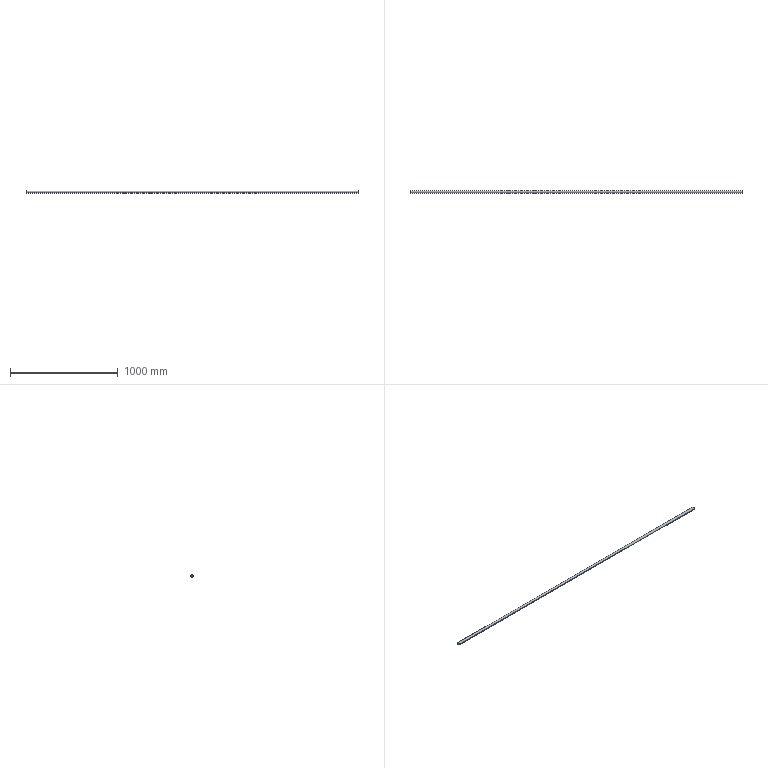Part | STEP file | 电柜护栏2栏杆_Default<As Machined> | 1 solid | 6 faces | box 3080 x 25 x 25 mm | volume 341083 mm3 | cylinder 4 | plane 2 | commonest cylinder face diameters 22 x2 25 x2
STEP:
#1=CARTESIAN_POINT('',(0.,0.,0.));
#2=DIRECTION('',(0.,0.,1.));
#3=DIRECTION('',(1.,0.,0.));
#4=AXIS2_PLACEMENT_3D('',#1,#2,#3);
#5=CARTESIAN_POINT('',(1540.,12.5,0.));
#6=VERTEX_POINT('',#5);
#7=CARTESIAN_POINT('',(1540.,-12.5,0.));
#8=VERTEX_POINT('',#7);
#9=CARTESIAN_POINT('',(1540.,0.,0.));
#10=DIRECTION('',(1.,0.,0.));
#11=DIRECTION('',(0.,1.,0.));
#12=AXIS2_PLACEMENT_3D('',#9,#10,#11);
#13=CIRCLE('',#12,12.5);
#14=CARTESIAN_POINT('',(1540.,0.,0.));
#15=DIRECTION('',(-1.,0.,0.));
#16=DIRECTION('',(0.,-1.,0.));
#17=AXIS2_PLACEMENT_3D('',#14,#15,#16);
#18=CYLINDRICAL_SURFACE('',#17,12.5);
#19=CARTESIAN_POINT('',(3.142,0.));
#20=DIRECTION('',(-1.,0.));
#21=VECTOR('',#20,1.);
#22=LINE('',#19,#21);
#23=(GEOMETRIC_REPRESENTATION_CONTEXT(2)PARAMETRIC_REPRESENTATION_CONTEXT()REPRESENTATION_CONTEXT('',''));
#24=DEFINITIONAL_REPRESENTATION('',(#22),#23);
#25=PCURVE('',#18,#24);
#26=CARTESIAN_POINT('',(1540.,0.,0.));
#27=DIRECTION('',(1.,0.,0.));
#28=DIRECTION('',(0.,1.,0.));
#29=AXIS2_PLACEMENT_3D('',#26,#27,#28);
#30=PLANE('',#29);
#31=CARTESIAN_POINT('',(0.,0.));
#32=DIRECTION('',(1.,0.));
#33=AXIS2_PLACEMENT_2D('',#31,#32);
#34=CIRCLE('',#33,12.5);
#35=(GEOMETRIC_REPRESENTATION_CONTEXT(2)PARAMETRIC_REPRESENTATION_CONTEXT()REPRESENTATION_CONTEXT('',''));
#36=DEFINITIONAL_REPRESENTATION('',(#34),#35);
#37=PCURVE('',#30,#36);
#38=SURFACE_CURVE('',#13,(#25,#37),.PCURVE_S1.);
#39=EDGE_CURVE('',#6,#8,#38,.T.);
#40=ORIENTED_EDGE('',*,*,#39,.F.);
#41=CARTESIAN_POINT('',(-1540.,12.5,0.));
#42=VERTEX_POINT('',#41);
#43=CARTESIAN_POINT('',(1540.,12.5,0.));
#44=DIRECTION('',(-1.,0.,0.));
#45=VECTOR('',#44,1.);
#46=LINE('',#43,#45);
#47=CARTESIAN_POINT('',(3.142,0.));
#48=DIRECTION('',(0.,1.));
#49=VECTOR('',#48,1.);
#50=LINE('',#47,#49);
#51=(GEOMETRIC_REPRESENTATION_CONTEXT(2)PARAMETRIC_REPRESENTATION_CONTEXT()REPRESENTATION_CONTEXT('',''));
#52=DEFINITIONAL_REPRESENTATION('',(#50),#51);
#53=PCURVE('',#18,#52);
#54=CARTESIAN_POINT('',(1540.,0.,0.));
#55=DIRECTION('',(-1.,0.,0.));
#56=DIRECTION('',(0.,-1.,0.));
#57=AXIS2_PLACEMENT_3D('',#54,#55,#56);
#58=CYLINDRICAL_SURFACE('',#57,12.5);
#59=CARTESIAN_POINT('',(3.142,0.));
#60=DIRECTION('',(0.,1.));
#61=VECTOR('',#60,1.);
#62=LINE('',#59,#61);
#63=(GEOMETRIC_REPRESENTATION_CONTEXT(2)PARAMETRIC_REPRESENTATION_CONTEXT()REPRESENTATION_CONTEXT('',''));
#64=DEFINITIONAL_REPRESENTATION('',(#62),#63);
#65=PCURVE('',#58,#64);
#66=SURFACE_CURVE('',#46,(#53,#65),.PCURVE_S1.);
#67=EDGE_CURVE('',#6,#42,#66,.T.);
#68=ORIENTED_EDGE('',*,*,#67,.T.);
#69=CARTESIAN_POINT('',(-1540.,-12.5,0.));
#70=VERTEX_POINT('',#69);
#71=CARTESIAN_POINT('',(-1540.,0.,0.));
#72=DIRECTION('',(1.,0.,0.));
#73=DIRECTION('',(0.,1.,0.));
#74=AXIS2_PLACEMENT_3D('',#71,#72,#73);
#75=CIRCLE('',#74,12.5);
#76=CARTESIAN_POINT('',(3.142,3080.));
#77=DIRECTION('',(-1.,0.));
#78=VECTOR('',#77,1.);
#79=LINE('',#76,#78);
#80=(GEOMETRIC_REPRESENTATION_CONTEXT(2)PARAMETRIC_REPRESENTATION_CONTEXT()REPRESENTATION_CONTEXT('',''));
#81=DEFINITIONAL_REPRESENTATION('',(#79),#80);
#82=PCURVE('',#18,#81);
#83=CARTESIAN_POINT('',(-1540.,0.,0.));
#84=DIRECTION('',(1.,0.,0.));
#85=DIRECTION('',(0.,1.,0.));
#86=AXIS2_PLACEMENT_3D('',#83,#84,#85);
#87=PLANE('',#86);
#88=CARTESIAN_POINT('',(0.,0.));
#89=DIRECTION('',(1.,0.));
#90=AXIS2_PLACEMENT_2D('',#88,#89);
#91=CIRCLE('',#90,12.5);
#92=(GEOMETRIC_REPRESENTATION_CONTEXT(2)PARAMETRIC_REPRESENTATION_CONTEXT()REPRESENTATION_CONTEXT('',''));
#93=DEFINITIONAL_REPRESENTATION('',(#91),#92);
#94=PCURVE('',#87,#93);
#95=SURFACE_CURVE('',#75,(#82,#94),.PCURVE_S1.);
#96=EDGE_CURVE('',#42,#70,#95,.T.);
#97=ORIENTED_EDGE('',*,*,#96,.T.);
#98=CARTESIAN_POINT('',(1540.,-12.5,0.));
#99=DIRECTION('',(-1.,0.,0.));
#100=VECTOR('',#99,1.);
#101=LINE('',#98,#100);
#102=CARTESIAN_POINT('',(0.,0.));
#103=DIRECTION('',(0.,1.));
#104=VECTOR('',#103,1.);
#105=LINE('',#102,#104);
#106=(GEOMETRIC_REPRESENTATION_CONTEXT(2)PARAMETRIC_REPRESENTATION_CONTEXT()REPRESENTATION_CONTEXT('',''));
#107=DEFINITIONAL_REPRESENTATION('',(#105),#106);
#108=PCURVE('',#18,#107);
#109=CARTESIAN_POINT('',(6.283,0.));
#110=DIRECTION('',(0.,1.));
#111=VECTOR('',#110,1.);
#112=LINE('',#109,#111);
#113=(GEOMETRIC_REPRESENTATION_CONTEXT(2)PARAMETRIC_REPRESENTATION_CONTEXT()REPRESENTATION_CONTEXT('',''));
#114=DEFINITIONAL_REPRESENTATION('',(#112),#113);
#115=PCURVE('',#58,#114);
#116=SURFACE_CURVE('',#101,(#108,#115),.PCURVE_S1.);
#117=EDGE_CURVE('',#8,#70,#116,.T.);
#118=ORIENTED_EDGE('',*,*,#117,.F.);
#119=EDGE_LOOP('',(#40,#68,#97,#118));
#120=FACE_BOUND('',#119,.T.);
#121=ADVANCED_FACE('',(#120),#18,.T.);
#122=CARTESIAN_POINT('',(1540.,-11.,0.));
#123=VERTEX_POINT('',#122);
#124=CARTESIAN_POINT('',(-1540.,-11.,0.));
#125=VERTEX_POINT('',#124);
#126=CARTESIAN_POINT('',(1540.,-11.,0.));
#127=DIRECTION('',(-1.,0.,0.));
#128=VECTOR('',#127,1.);
#129=LINE('',#126,#128);
#130=CARTESIAN_POINT('',(1540.,0.,0.));
#131=DIRECTION('',(-1.,0.,0.));
#132=DIRECTION('',(0.,-1.,0.));
#133=AXIS2_PLACEMENT_3D('',#130,#131,#132);
#134=CYLINDRICAL_SURFACE('',#133,11.);
#135=CARTESIAN_POINT('',(6.283,0.));
#136=DIRECTION('',(0.,1.));
#137=VECTOR('',#136,1.);
#138=LINE('',#135,#137);
#139=(GEOMETRIC_REPRESENTATION_CONTEXT(2)PARAMETRIC_REPRESENTATION_CONTEXT()REPRESENTATION_CONTEXT('',''));
#140=DEFINITIONAL_REPRESENTATION('',(#138),#139);
#141=PCURVE('',#134,#140);
#142=CARTESIAN_POINT('',(1540.,0.,0.));
#143=DIRECTION('',(-1.,0.,0.));
#144=DIRECTION('',(0.,-1.,0.));
#145=AXIS2_PLACEMENT_3D('',#142,#143,#144);
#146=CYLINDRICAL_SURFACE('',#145,11.);
#147=CARTESIAN_POINT('',(0.,0.));
#148=DIRECTION('',(0.,1.));
#149=VECTOR('',#148,1.);
#150=LINE('',#147,#149);
#151=(GEOMETRIC_REPRESENTATION_CONTEXT(2)PARAMETRIC_REPRESENTATION_CONTEXT()REPRESENTATION_CONTEXT('',''));
#152=DEFINITIONAL_REPRESENTATION('',(#150),#151);
#153=PCURVE('',#146,#152);
#154=SURFACE_CURVE('',#129,(#141,#153),.PCURVE_S1.);
#155=EDGE_CURVE('',#123,#125,#154,.T.);
#156=ORIENTED_EDGE('',*,*,#155,.T.);
#157=CARTESIAN_POINT('',(-1540.,11.,0.));
#158=VERTEX_POINT('',#157);
#159=CARTESIAN_POINT('',(-1540.,0.,0.));
#160=DIRECTION('',(1.,0.,0.));
#161=DIRECTION('',(0.,1.,0.));
#162=AXIS2_PLACEMENT_3D('',#159,#160,#161);
#163=CIRCLE('',#162,11.);
#164=CARTESIAN_POINT('',(9.425,3080.));
#165=DIRECTION('',(-1.,0.));
#166=VECTOR('',#165,1.);
#167=LINE('',#164,#166);
#168=(GEOMETRIC_REPRESENTATION_CONTEXT(2)PARAMETRIC_REPRESENTATION_CONTEXT()REPRESENTATION_CONTEXT('',''));
#169=DEFINITIONAL_REPRESENTATION('',(#167),#168);
#170=PCURVE('',#134,#169);
#171=CARTESIAN_POINT('',(0.,0.));
#172=DIRECTION('',(1.,0.));
#173=AXIS2_PLACEMENT_2D('',#171,#172);
#174=CIRCLE('',#173,11.);
#175=(GEOMETRIC_REPRESENTATION_CONTEXT(2)PARAMETRIC_REPRESENTATION_CONTEXT()REPRESENTATION_CONTEXT('',''));
#176=DEFINITIONAL_REPRESENTATION('',(#174),#175);
#177=PCURVE('',#87,#176);
#178=SURFACE_CURVE('',#163,(#170,#177),.PCURVE_S1.);
#179=EDGE_CURVE('',#125,#158,#178,.T.);
#180=ORIENTED_EDGE('',*,*,#179,.T.);
#181=CARTESIAN_POINT('',(1540.,11.,0.));
#182=VERTEX_POINT('',#181);
#183=CARTESIAN_POINT('',(1540.,11.,0.));
#184=DIRECTION('',(-1.,0.,0.));
#185=VECTOR('',#184,1.);
#186=LINE('',#183,#185);
#187=CARTESIAN_POINT('',(3.142,0.));
#188=DIRECTION('',(0.,1.));
#189=VECTOR('',#188,1.);
#190=LINE('',#187,#189);
#191=(GEOMETRIC_REPRESENTATION_CONTEXT(2)PARAMETRIC_REPRESENTATION_CONTEXT()REPRESENTATION_CONTEXT('',''));
#192=DEFINITIONAL_REPRESENTATION('',(#190),#191);
#193=PCURVE('',#134,#192);
#194=CARTESIAN_POINT('',(3.142,0.));
#195=DIRECTION('',(0.,1.));
#196=VECTOR('',#195,1.);
#197=LINE('',#194,#196);
#198=(GEOMETRIC_REPRESENTATION_CONTEXT(2)PARAMETRIC_REPRESENTATION_CONTEXT()REPRESENTATION_CONTEXT('',''));
#199=DEFINITIONAL_REPRESENTATION('',(#197),#198);
#200=PCURVE('',#146,#199);
#201=SURFACE_CURVE('',#186,(#193,#200),.PCURVE_S1.);
#202=EDGE_CURVE('',#182,#158,#201,.T.);
#203=ORIENTED_EDGE('',*,*,#202,.F.);
#204=CARTESIAN_POINT('',(1540.,0.,0.));
#205=DIRECTION('',(1.,0.,0.));
#206=DIRECTION('',(0.,1.,0.));
#207=AXIS2_PLACEMENT_3D('',#204,#205,#206);
#208=CIRCLE('',#207,11.);
#209=CARTESIAN_POINT('',(9.425,0.));
#210=DIRECTION('',(-1.,0.));
#211=VECTOR('',#210,1.);
#212=LINE('',#209,#211);
#213=(GEOMETRIC_REPRESENTATION_CONTEXT(2)PARAMETRIC_REPRESENTATION_CONTEXT()REPRESENTATION_CONTEXT('',''));
#214=DEFINITIONAL_REPRESENTATION('',(#212),#213);
#215=PCURVE('',#134,#214);
#216=CARTESIAN_POINT('',(0.,0.));
#217=DIRECTION('',(1.,0.));
#218=AXIS2_PLACEMENT_2D('',#216,#217);
#219=CIRCLE('',#218,11.);
#220=(GEOMETRIC_REPRESENTATION_CONTEXT(2)PARAMETRIC_REPRESENTATION_CONTEXT()REPRESENTATION_CONTEXT('',''));
#221=DEFINITIONAL_REPRESENTATION('',(#219),#220);
#222=PCURVE('',#30,#221);
#223=SURFACE_CURVE('',#208,(#215,#222),.PCURVE_S1.);
#224=EDGE_CURVE('',#123,#182,#223,.T.);
#225=ORIENTED_EDGE('',*,*,#224,.F.);
#226=EDGE_LOOP('',(#156,#180,#203,#225));
#227=FACE_BOUND('',#226,.F.);
#228=ADVANCED_FACE('',(#227),#134,.F.);
#229=CARTESIAN_POINT('',(-1540.,0.,0.));
#230=DIRECTION('',(1.,0.,0.));
#231=DIRECTION('',(0.,1.,0.));
#232=AXIS2_PLACEMENT_3D('',#229,#230,#231);
#233=CIRCLE('',#232,11.);
#234=CARTESIAN_POINT('',(3.142,3080.));
#235=DIRECTION('',(-1.,0.));
#236=VECTOR('',#235,1.);
#237=LINE('',#234,#236);
#238=(GEOMETRIC_REPRESENTATION_CONTEXT(2)PARAMETRIC_REPRESENTATION_CONTEXT()REPRESENTATION_CONTEXT('',''));
#239=DEFINITIONAL_REPRESENTATION('',(#237),#238);
#240=PCURVE('',#146,#239);
#241=CARTESIAN_POINT('',(0.,0.));
#242=DIRECTION('',(1.,0.));
#243=AXIS2_PLACEMENT_2D('',#241,#242);
#244=CIRCLE('',#243,11.);
#245=(GEOMETRIC_REPRESENTATION_CONTEXT(2)PARAMETRIC_REPRESENTATION_CONTEXT()REPRESENTATION_CONTEXT('',''));
#246=DEFINITIONAL_REPRESENTATION('',(#244),#245);
#247=PCURVE('',#87,#246);
#248=SURFACE_CURVE('',#233,(#240,#247),.PCURVE_S1.);
#249=EDGE_CURVE('',#158,#125,#248,.T.);
#250=ORIENTED_EDGE('',*,*,#249,.T.);
#251=ORIENTED_EDGE('',*,*,#155,.F.);
#252=CARTESIAN_POINT('',(1540.,0.,0.));
#253=DIRECTION('',(1.,0.,0.));
#254=DIRECTION('',(0.,1.,0.));
#255=AXIS2_PLACEMENT_3D('',#252,#253,#254);
#256=CIRCLE('',#255,11.);
#257=CARTESIAN_POINT('',(3.142,0.));
#258=DIRECTION('',(-1.,0.));
#259=VECTOR('',#258,1.);
#260=LINE('',#257,#259);
#261=(GEOMETRIC_REPRESENTATION_CONTEXT(2)PARAMETRIC_REPRESENTATION_CONTEXT()REPRESENTATION_CONTEXT('',''));
#262=DEFINITIONAL_REPRESENTATION('',(#260),#261);
#263=PCURVE('',#146,#262);
#264=CARTESIAN_POINT('',(0.,0.));
#265=DIRECTION('',(1.,0.));
#266=AXIS2_PLACEMENT_2D('',#264,#265);
#267=CIRCLE('',#266,11.);
#268=(GEOMETRIC_REPRESENTATION_CONTEXT(2)PARAMETRIC_REPRESENTATION_CONTEXT()REPRESENTATION_CONTEXT('',''));
#269=DEFINITIONAL_REPRESENTATION('',(#267),#268);
#270=PCURVE('',#30,#269);
#271=SURFACE_CURVE('',#256,(#263,#270),.PCURVE_S1.);
#272=EDGE_CURVE('',#182,#123,#271,.T.);
#273=ORIENTED_EDGE('',*,*,#272,.F.);
#274=ORIENTED_EDGE('',*,*,#202,.T.);
#275=EDGE_LOOP('',(#250,#251,#273,#274));
#276=FACE_BOUND('',#275,.F.);
#277=ADVANCED_FACE('',(#276),#146,.F.);
#278=ORIENTED_EDGE('',*,*,#67,.F.);
#279=CARTESIAN_POINT('',(1540.,0.,0.));
#280=DIRECTION('',(1.,0.,0.));
#281=DIRECTION('',(0.,1.,0.));
#282=AXIS2_PLACEMENT_3D('',#279,#280,#281);
#283=CIRCLE('',#282,12.5);
#284=CARTESIAN_POINT('',(9.425,0.));
#285=DIRECTION('',(-1.,0.));
#286=VECTOR('',#285,1.);
#287=LINE('',#284,#286);
#288=(GEOMETRIC_REPRESENTATION_CONTEXT(2)PARAMETRIC_REPRESENTATION_CONTEXT()REPRESENTATION_CONTEXT('',''));
#289=DEFINITIONAL_REPRESENTATION('',(#287),#288);
#290=PCURVE('',#58,#289);
#291=CARTESIAN_POINT('',(0.,0.));
#292=DIRECTION('',(1.,0.));
#293=AXIS2_PLACEMENT_2D('',#291,#292);
#294=CIRCLE('',#293,12.5);
#295=(GEOMETRIC_REPRESENTATION_CONTEXT(2)PARAMETRIC_REPRESENTATION_CONTEXT()REPRESENTATION_CONTEXT('',''));
#296=DEFINITIONAL_REPRESENTATION('',(#294),#295);
#297=PCURVE('',#30,#296);
#298=SURFACE_CURVE('',#283,(#290,#297),.PCURVE_S1.);
#299=EDGE_CURVE('',#8,#6,#298,.T.);
#300=ORIENTED_EDGE('',*,*,#299,.F.);
#301=ORIENTED_EDGE('',*,*,#117,.T.);
#302=CARTESIAN_POINT('',(-1540.,0.,0.));
#303=DIRECTION('',(1.,0.,0.));
#304=DIRECTION('',(0.,1.,0.));
#305=AXIS2_PLACEMENT_3D('',#302,#303,#304);
#306=CIRCLE('',#305,12.5);
#307=CARTESIAN_POINT('',(9.425,3080.));
#308=DIRECTION('',(-1.,0.));
#309=VECTOR('',#308,1.);
#310=LINE('',#307,#309);
#311=(GEOMETRIC_REPRESENTATION_CONTEXT(2)PARAMETRIC_REPRESENTATION_CONTEXT()REPRESENTATION_CONTEXT('',''));
#312=DEFINITIONAL_REPRESENTATION('',(#310),#311);
#313=PCURVE('',#58,#312);
#314=CARTESIAN_POINT('',(0.,0.));
#315=DIRECTION('',(1.,0.));
#316=AXIS2_PLACEMENT_2D('',#314,#315);
#317=CIRCLE('',#316,12.5);
#318=(GEOMETRIC_REPRESENTATION_CONTEXT(2)PARAMETRIC_REPRESENTATION_CONTEXT()REPRESENTATION_CONTEXT('',''));
#319=DEFINITIONAL_REPRESENTATION('',(#317),#318);
#320=PCURVE('',#87,#319);
#321=SURFACE_CURVE('',#306,(#313,#320),.PCURVE_S1.);
#322=EDGE_CURVE('',#70,#42,#321,.T.);
#323=ORIENTED_EDGE('',*,*,#322,.T.);
#324=EDGE_LOOP('',(#278,#300,#301,#323));
#325=FACE_BOUND('',#324,.T.);
#326=ADVANCED_FACE('',(#325),#58,.T.);
#327=ORIENTED_EDGE('',*,*,#224,.F.);
#328=ORIENTED_EDGE('',*,*,#272,.F.);
#329=EDGE_LOOP('',(#327,#328));
#330=FACE_BOUND('',#329,.T.);
#331=ORIENTED_EDGE('',*,*,#299,.T.);
#332=ORIENTED_EDGE('',*,*,#39,.T.);
#333=EDGE_LOOP('',(#331,#332));
#334=FACE_BOUND('',#333,.T.);
#335=ADVANCED_FACE('',(#330,#334),#30,.T.);
#336=ORIENTED_EDGE('',*,*,#179,.T.);
#337=ORIENTED_EDGE('',*,*,#249,.T.);
#338=EDGE_LOOP('',(#336,#337));
#339=FACE_BOUND('',#338,.T.);
#340=ORIENTED_EDGE('',*,*,#322,.F.);
#341=ORIENTED_EDGE('',*,*,#96,.F.);
#342=EDGE_LOOP('',(#340,#341));
#343=FACE_BOUND('',#342,.T.);
#344=ADVANCED_FACE('',(#339,#343),#87,.F.);
#345=CLOSED_SHELL('',(#121,#228,#277,#326,#335,#344));
#346=MANIFOLD_SOLID_BREP('',#345);
#347=(LENGTH_UNIT()NAMED_UNIT(*)SI_UNIT(.MILLI.,.METRE.));
#348=UNCERTAINTY_MEASURE_WITH_UNIT(LENGTH_MEASURE(0.0000001),#347,'','');
#349=(NAMED_UNIT(*)PLANE_ANGLE_UNIT()SI_UNIT($,.RADIAN.));
#350=(NAMED_UNIT(*)SI_UNIT($,.STERADIAN.)SOLID_ANGLE_UNIT());
#351=(GEOMETRIC_REPRESENTATION_CONTEXT(3)GLOBAL_UNCERTAINTY_ASSIGNED_CONTEXT((#348))GLOBAL_UNIT_ASSIGNED_CONTEXT((#347,#349,#350))REPRESENTATION_CONTEXT('',''));
#352=ADVANCED_BREP_SHAPE_REPRESENTATION('',(#4,#346),#351);